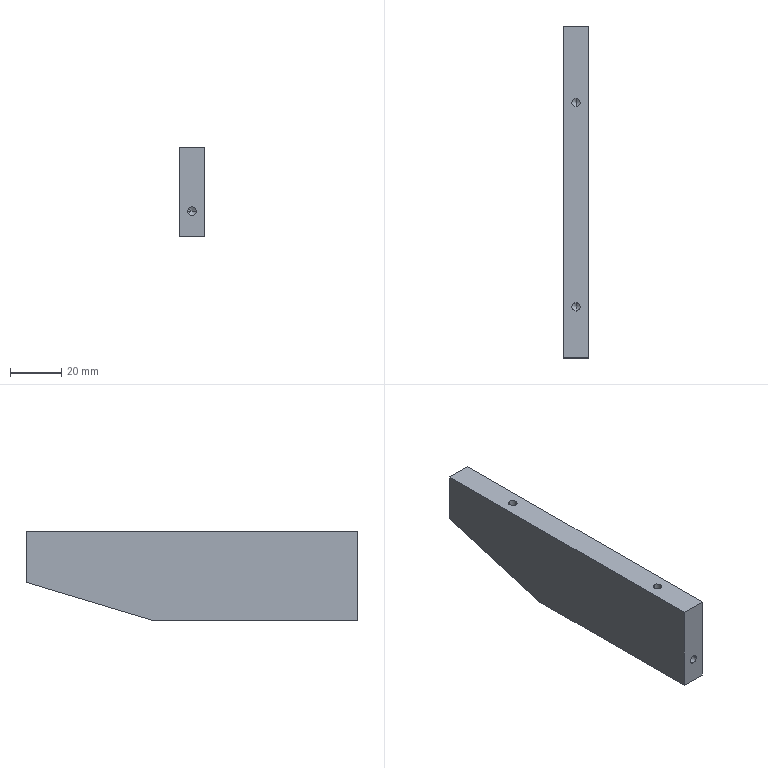Part | STEP file | 04-14 Guide reinforcing rib | 1 solid | 19 faces | box 10 x 130 x 35 mm | volume 41228 mm3 | plane 7 | cylinder 6 | cone 6 | commonest cylinder face diameters 3.3 x6
STEP:
#1=CARTESIAN_POINT('',(0.,0.,0.));
#2=DIRECTION('',(0.,0.,1.));
#3=DIRECTION('',(1.,0.,0.));
#4=AXIS2_PLACEMENT_3D('',#1,#2,#3);
#5=CARTESIAN_POINT('',(0.,18.35,-20.));
#6=VERTEX_POINT('',#5);
#7=CARTESIAN_POINT('',(0.,18.35,0.));
#8=VERTEX_POINT('',#7);
#9=CARTESIAN_POINT('',(0.,18.35,-20.));
#10=DIRECTION('',(0.,0.,1.));
#11=VECTOR('',#10,1.);
#12=LINE('',#9,#11);
#13=CARTESIAN_POINT('',(0.,20.,-20.));
#14=DIRECTION('',(0.,0.,1.));
#15=DIRECTION('',(0.,-1.,0.));
#16=AXIS2_PLACEMENT_3D('',#13,#14,#15);
#17=CYLINDRICAL_SURFACE('',#16,1.65);
#18=CARTESIAN_POINT('',(6.283,0.));
#19=DIRECTION('',(0.,1.));
#20=VECTOR('',#19,1.);
#21=LINE('',#18,#20);
#22=(GEOMETRIC_REPRESENTATION_CONTEXT(2)PARAMETRIC_REPRESENTATION_CONTEXT()REPRESENTATION_CONTEXT('',''));
#23=DEFINITIONAL_REPRESENTATION('',(#21),#22);
#24=PCURVE('',#17,#23);
#25=CARTESIAN_POINT('',(0.,20.,-20.));
#26=DIRECTION('',(0.,0.,1.));
#27=DIRECTION('',(0.,-1.,0.));
#28=AXIS2_PLACEMENT_3D('',#25,#26,#27);
#29=CYLINDRICAL_SURFACE('',#28,1.65);
#30=CARTESIAN_POINT('',(0.,0.));
#31=DIRECTION('',(0.,1.));
#32=VECTOR('',#31,1.);
#33=LINE('',#30,#32);
#34=(GEOMETRIC_REPRESENTATION_CONTEXT(2)PARAMETRIC_REPRESENTATION_CONTEXT()REPRESENTATION_CONTEXT('',''));
#35=DEFINITIONAL_REPRESENTATION('',(#33),#34);
#36=PCURVE('',#29,#35);
#37=SURFACE_CURVE('',#12,(#24,#36),.PCURVE_S1.);
#38=EDGE_CURVE('',#6,#8,#37,.T.);
#39=ORIENTED_EDGE('',*,*,#38,.T.);
#40=CARTESIAN_POINT('',(0.,21.65,0.));
#41=VERTEX_POINT('',#40);
#42=CARTESIAN_POINT('',(0.,20.,0.));
#43=DIRECTION('',(0.,0.,1.));
#44=DIRECTION('',(0.,-1.,0.));
#45=AXIS2_PLACEMENT_3D('',#42,#43,#44);
#46=CIRCLE('',#45,1.65);
#47=CARTESIAN_POINT('',(0.,20.));
#48=DIRECTION('',(1.,0.));
#49=VECTOR('',#48,1.);
#50=LINE('',#47,#49);
#51=(GEOMETRIC_REPRESENTATION_CONTEXT(2)PARAMETRIC_REPRESENTATION_CONTEXT()REPRESENTATION_CONTEXT('',''));
#52=DEFINITIONAL_REPRESENTATION('',(#50),#51);
#53=PCURVE('',#17,#52);
#54=CARTESIAN_POINT('',(5.,0.,0.));
#55=DIRECTION('',(0.,0.,-1.));
#56=DIRECTION('',(-1.,0.,0.));
#57=AXIS2_PLACEMENT_3D('',#54,#55,#56);
#58=PLANE('',#57);
#59=CARTESIAN_POINT('',(5.,18.35));
#60=CARTESIAN_POINT('',(2.142,18.35));
#61=CARTESIAN_POINT('',(3.571,20.825));
#62=CARTESIAN_POINT('',(5.,23.3));
#63=CARTESIAN_POINT('',(6.429,20.825));
#64=CARTESIAN_POINT('',(7.858,18.35));
#65=CARTESIAN_POINT('',(5.,18.35));
#66=(BOUNDED_CURVE()B_SPLINE_CURVE(2,(#59,#60,#61,#62,#63,#64,#65),.UNSPECIFIED.,.T.,.F.)B_SPLINE_CURVE_WITH_KNOTS((1,2,2,2,2,1),(-2.094,0.,2.094,4.189,6.283,8.378),.UNSPECIFIED.)CURVE()GEOMETRIC_REPRESENTATION_ITEM()RATIONAL_B_SPLINE_CURVE((1.,0.5,1.,0.5,1.,0.5,1.))REPRESENTATION_ITEM(''));
#67=(GEOMETRIC_REPRESENTATION_CONTEXT(2)PARAMETRIC_REPRESENTATION_CONTEXT()REPRESENTATION_CONTEXT('',''));
#68=DEFINITIONAL_REPRESENTATION('',(#66),#67);
#69=PCURVE('',#58,#68);
#70=SURFACE_CURVE('',#46,(#53,#69),.PCURVE_S1.);
#71=EDGE_CURVE('',#41,#8,#70,.T.);
#72=ORIENTED_EDGE('',*,*,#71,.F.);
#73=CARTESIAN_POINT('',(0.,21.65,-20.));
#74=VERTEX_POINT('',#73);
#75=CARTESIAN_POINT('',(0.,21.65,-20.));
#76=DIRECTION('',(0.,0.,1.));
#77=VECTOR('',#76,1.);
#78=LINE('',#75,#77);
#79=CARTESIAN_POINT('',(3.142,0.));
#80=DIRECTION('',(0.,1.));
#81=VECTOR('',#80,1.);
#82=LINE('',#79,#81);
#83=(GEOMETRIC_REPRESENTATION_CONTEXT(2)PARAMETRIC_REPRESENTATION_CONTEXT()REPRESENTATION_CONTEXT('',''));
#84=DEFINITIONAL_REPRESENTATION('',(#82),#83);
#85=PCURVE('',#17,#84);
#86=CARTESIAN_POINT('',(3.142,0.));
#87=DIRECTION('',(0.,1.));
#88=VECTOR('',#87,1.);
#89=LINE('',#86,#88);
#90=(GEOMETRIC_REPRESENTATION_CONTEXT(2)PARAMETRIC_REPRESENTATION_CONTEXT()REPRESENTATION_CONTEXT('',''));
#91=DEFINITIONAL_REPRESENTATION('',(#89),#90);
#92=PCURVE('',#29,#91);
#93=SURFACE_CURVE('',#78,(#85,#92),.PCURVE_S1.);
#94=EDGE_CURVE('',#74,#41,#93,.T.);
#95=ORIENTED_EDGE('',*,*,#94,.F.);
#96=CARTESIAN_POINT('',(0.,20.,-20.));
#97=DIRECTION('',(0.,0.,-1.));
#98=DIRECTION('',(1.,0.,0.));
#99=AXIS2_PLACEMENT_3D('',#96,#97,#98);
#100=CIRCLE('',#99,1.65);
#101=CARTESIAN_POINT('',(7.854,0.));
#102=DIRECTION('',(-1.,0.));
#103=VECTOR('',#102,1.);
#104=LINE('',#101,#103);
#105=(GEOMETRIC_REPRESENTATION_CONTEXT(2)PARAMETRIC_REPRESENTATION_CONTEXT()REPRESENTATION_CONTEXT('',''));
#106=DEFINITIONAL_REPRESENTATION('',(#104),#105);
#107=PCURVE('',#17,#106);
#108=CARTESIAN_POINT('',(0.,20.,979.009));
#109=DIRECTION('',(0.,0.,1.));
#110=DIRECTION('',(0.,-1.,0.));
#111=AXIS2_PLACEMENT_3D('',#108,#109,#110);
#112=CONICAL_SURFACE('',#111,1664.279,1.03);
#113=CARTESIAN_POINT('',(7.854,-999.009));
#114=DIRECTION('',(-1.,0.));
#115=VECTOR('',#114,1.);
#116=LINE('',#113,#115);
#117=(GEOMETRIC_REPRESENTATION_CONTEXT(2)PARAMETRIC_REPRESENTATION_CONTEXT()REPRESENTATION_CONTEXT('',''));
#118=DEFINITIONAL_REPRESENTATION('',(#116),#117);
#119=PCURVE('',#112,#118);
#120=SURFACE_CURVE('',#100,(#107,#119),.PCURVE_S1.);
#121=EDGE_CURVE('',#6,#74,#120,.T.);
#122=ORIENTED_EDGE('',*,*,#121,.F.);
#123=EDGE_LOOP('',(#39,#72,#95,#122));
#124=FACE_BOUND('',#123,.F.);
#125=ADVANCED_FACE('',(#124),#17,.F.);
#126=ORIENTED_EDGE('',*,*,#121,.T.);
#127=CARTESIAN_POINT('',(0.,20.,-20.991));
#128=VERTEX_POINT('',#127);
#129=CARTESIAN_POINT('',(0.,20.,-20.991));
#130=DIRECTION('',(0.,0.8572,0.515));
#131=VECTOR('',#130,1.);
#132=LINE('',#129,#131);
#133=CARTESIAN_POINT('',(3.142,-1000.));
#134=CARTESIAN_POINT('',(3.142,-999.985));
#135=CARTESIAN_POINT('',(3.142,-999.955));
#136=CARTESIAN_POINT('',(3.142,-999.91));
#137=CARTESIAN_POINT('',(3.142,-999.865));
#138=CARTESIAN_POINT('',(3.142,-999.82));
#139=CARTESIAN_POINT('',(3.142,-999.775));
#140=CARTESIAN_POINT('',(3.142,-999.73));
#141=CARTESIAN_POINT('',(3.142,-999.685));
#142=CARTESIAN_POINT('',(3.142,-999.639));
#143=CARTESIAN_POINT('',(3.142,-999.594));
#144=CARTESIAN_POINT('',(3.142,-999.549));
#145=CARTESIAN_POINT('',(3.142,-999.504));
#146=CARTESIAN_POINT('',(3.142,-999.459));
#147=CARTESIAN_POINT('',(3.142,-999.414));
#148=CARTESIAN_POINT('',(3.142,-999.369));
#149=CARTESIAN_POINT('',(3.142,-999.324));
#150=CARTESIAN_POINT('',(3.142,-999.279));
#151=CARTESIAN_POINT('',(3.142,-999.234));
#152=CARTESIAN_POINT('',(3.142,-999.189));
#153=CARTESIAN_POINT('',(3.142,-999.144));
#154=CARTESIAN_POINT('',(3.142,-999.099));
#155=CARTESIAN_POINT('',(3.142,-999.054));
#156=CARTESIAN_POINT('',(3.142,-999.024));
#157=CARTESIAN_POINT('',(3.142,-999.009));
#158=B_SPLINE_CURVE_WITH_KNOTS('',3,(#133,#134,#135,#136,#137,#138,#139,#140,#141,#142,#143,#144,#145,#146,#147,#148,#149,#150,#151,#152,#153,#154,#155,#156,#157),.UNSPECIFIED.,.F.,.F.,(4,1,1,1,1,1,1,1,1,1,1,1,1,1,1,1,1,1,1,1,1,1,4),(0.,0.0875,0.175,0.2625,0.35,0.4375,0.525,0.6125,0.7,0.7875,0.875,0.9625,1.05,1.137,1.225,1.312,1.4,1.487,1.575,1.662,1.75,1.837,1.925),.QUASI_UNIFORM_KNOTS.);
#159=(GEOMETRIC_REPRESENTATION_CONTEXT(2)PARAMETRIC_REPRESENTATION_CONTEXT()REPRESENTATION_CONTEXT('',''));
#160=DEFINITIONAL_REPRESENTATION('',(#158),#159);
#161=PCURVE('',#112,#160);
#162=CARTESIAN_POINT('',(0.,20.,979.009));
#163=DIRECTION('',(0.,0.,1.));
#164=DIRECTION('',(0.,-1.,0.));
#165=AXIS2_PLACEMENT_3D('',#162,#163,#164);
#166=CONICAL_SURFACE('',#165,1664.279,1.03);
#167=CARTESIAN_POINT('',(3.142,-1000.));
#168=CARTESIAN_POINT('',(3.142,-999.985));
#169=CARTESIAN_POINT('',(3.142,-999.955));
#170=CARTESIAN_POINT('',(3.142,-999.91));
#171=CARTESIAN_POINT('',(3.142,-999.865));
#172=CARTESIAN_POINT('',(3.142,-999.82));
#173=CARTESIAN_POINT('',(3.142,-999.775));
#174=CARTESIAN_POINT('',(3.142,-999.73));
#175=CARTESIAN_POINT('',(3.142,-999.685));
#176=CARTESIAN_POINT('',(3.142,-999.639));
#177=CARTESIAN_POINT('',(3.142,-999.594));
#178=CARTESIAN_POINT('',(3.142,-999.549));
#179=CARTESIAN_POINT('',(3.142,-999.504));
#180=CARTESIAN_POINT('',(3.142,-999.459));
#181=CARTESIAN_POINT('',(3.142,-999.414));
#182=CARTESIAN_POINT('',(3.142,-999.369));
#183=CARTESIAN_POINT('',(3.142,-999.324));
#184=CARTESIAN_POINT('',(3.142,-999.279));
#185=CARTESIAN_POINT('',(3.142,-999.234));
#186=CARTESIAN_POINT('',(3.142,-999.189));
#187=CARTESIAN_POINT('',(3.142,-999.144));
#188=CARTESIAN_POINT('',(3.142,-999.099));
#189=CARTESIAN_POINT('',(3.142,-999.054));
#190=CARTESIAN_POINT('',(3.142,-999.024));
#191=CARTESIAN_POINT('',(3.142,-999.009));
#192=B_SPLINE_CURVE_WITH_KNOTS('',3,(#167,#168,#169,#170,#171,#172,#173,#174,#175,#176,#177,#178,#179,#180,#181,#182,#183,#184,#185,#186,#187,#188,#189,#190,#191),.UNSPECIFIED.,.F.,.F.,(4,1,1,1,1,1,1,1,1,1,1,1,1,1,1,1,1,1,1,1,1,1,4),(0.,0.0875,0.175,0.2625,0.35,0.4375,0.525,0.6125,0.7,0.7875,0.875,0.9625,1.05,1.137,1.225,1.312,1.4,1.487,1.575,1.662,1.75,1.837,1.925),.QUASI_UNIFORM_KNOTS.);
#193=(GEOMETRIC_REPRESENTATION_CONTEXT(2)PARAMETRIC_REPRESENTATION_CONTEXT()REPRESENTATION_CONTEXT('',''));
#194=DEFINITIONAL_REPRESENTATION('',(#192),#193);
#195=PCURVE('',#166,#194);
#196=SURFACE_CURVE('',#132,(#161,#195),.PCURVE_S1.);
#197=EDGE_CURVE('',#128,#74,#196,.T.);
#198=ORIENTED_EDGE('',*,*,#197,.F.);
#199=CARTESIAN_POINT('',(0.,20.,-20.991));
#200=DIRECTION('',(0.,-0.8572,0.515));
#201=VECTOR('',#200,1.);
#202=LINE('',#199,#201);
#203=CARTESIAN_POINT('',(6.283,-1000.));
#204=DIRECTION('',(0.,1.));
#205=VECTOR('',#204,1.);
#206=LINE('',#203,#205);
#207=(GEOMETRIC_REPRESENTATION_CONTEXT(2)PARAMETRIC_REPRESENTATION_CONTEXT()REPRESENTATION_CONTEXT('',''));
#208=DEFINITIONAL_REPRESENTATION('',(#206),#207);
#209=PCURVE('',#112,#208);
#210=CARTESIAN_POINT('',(0.,-1000.));
#211=DIRECTION('',(0.,1.));
#212=VECTOR('',#211,1.);
#213=LINE('',#210,#212);
#214=(GEOMETRIC_REPRESENTATION_CONTEXT(2)PARAMETRIC_REPRESENTATION_CONTEXT()REPRESENTATION_CONTEXT('',''));
#215=DEFINITIONAL_REPRESENTATION('',(#213),#214);
#216=PCURVE('',#166,#215);
#217=SURFACE_CURVE('',#202,(#209,#216),.PCURVE_S1.);
#218=EDGE_CURVE('',#128,#6,#217,.T.);
#219=ORIENTED_EDGE('',*,*,#218,.T.);
#220=EDGE_LOOP('',(#126,#198,#219));
#221=FACE_BOUND('',#220,.F.);
#222=ADVANCED_FACE('',(#221),#112,.F.);
#223=CARTESIAN_POINT('',(0.,98.35,-20.));
#224=VERTEX_POINT('',#223);
#225=CARTESIAN_POINT('',(0.,98.35,0.));
#226=VERTEX_POINT('',#225);
#227=CARTESIAN_POINT('',(0.,98.35,-20.));
#228=DIRECTION('',(0.,0.,1.));
#229=VECTOR('',#228,1.);
#230=LINE('',#227,#229);
#231=CARTESIAN_POINT('',(0.,100.,-20.));
#232=DIRECTION('',(0.,0.,1.));
#233=DIRECTION('',(0.,-1.,0.));
#234=AXIS2_PLACEMENT_3D('',#231,#232,#233);
#235=CYLINDRICAL_SURFACE('',#234,1.65);
#236=CARTESIAN_POINT('',(6.283,0.));
#237=DIRECTION('',(0.,1.));
#238=VECTOR('',#237,1.);
#239=LINE('',#236,#238);
#240=(GEOMETRIC_REPRESENTATION_CONTEXT(2)PARAMETRIC_REPRESENTATION_CONTEXT()REPRESENTATION_CONTEXT('',''));
#241=DEFINITIONAL_REPRESENTATION('',(#239),#240);
#242=PCURVE('',#235,#241);
#243=CARTESIAN_POINT('',(0.,100.,-20.));
#244=DIRECTION('',(0.,0.,1.));
#245=DIRECTION('',(0.,-1.,0.));
#246=AXIS2_PLACEMENT_3D('',#243,#244,#245);
#247=CYLINDRICAL_SURFACE('',#246,1.65);
#248=CARTESIAN_POINT('',(0.,0.));
#249=DIRECTION('',(0.,1.));
#250=VECTOR('',#249,1.);
#251=LINE('',#248,#250);
#252=(GEOMETRIC_REPRESENTATION_CONTEXT(2)PARAMETRIC_REPRESENTATION_CONTEXT()REPRESENTATION_CONTEXT('',''));
#253=DEFINITIONAL_REPRESENTATION('',(#251),#252);
#254=PCURVE('',#247,#253);
#255=SURFACE_CURVE('',#230,(#242,#254),.PCURVE_S1.);
#256=EDGE_CURVE('',#224,#226,#255,.T.);
#257=ORIENTED_EDGE('',*,*,#256,.T.);
#258=CARTESIAN_POINT('',(0.,101.65,0.));
#259=VERTEX_POINT('',#258);
#260=CARTESIAN_POINT('',(0.,100.,0.));
#261=DIRECTION('',(0.,0.,1.));
#262=DIRECTION('',(0.,-1.,0.));
#263=AXIS2_PLACEMENT_3D('',#260,#261,#262);
#264=CIRCLE('',#263,1.65);
#265=CARTESIAN_POINT('',(0.,20.));
#266=DIRECTION('',(1.,0.));
#267=VECTOR('',#266,1.);
#268=LINE('',#265,#267);
#269=(GEOMETRIC_REPRESENTATION_CONTEXT(2)PARAMETRIC_REPRESENTATION_CONTEXT()REPRESENTATION_CONTEXT('',''));
#270=DEFINITIONAL_REPRESENTATION('',(#268),#269);
#271=PCURVE('',#235,#270);
#272=CARTESIAN_POINT('',(5.,98.35));
#273=CARTESIAN_POINT('',(2.142,98.35));
#274=CARTESIAN_POINT('',(3.571,100.825));
#275=CARTESIAN_POINT('',(5.,103.3));
#276=CARTESIAN_POINT('',(6.429,100.825));
#277=CARTESIAN_POINT('',(7.858,98.35));
#278=CARTESIAN_POINT('',(5.,98.35));
#279=(BOUNDED_CURVE()B_SPLINE_CURVE(2,(#272,#273,#274,#275,#276,#277,#278),.UNSPECIFIED.,.T.,.F.)B_SPLINE_CURVE_WITH_KNOTS((1,2,2,2,2,1),(-2.094,0.,2.094,4.189,6.283,8.378),.UNSPECIFIED.)CURVE()GEOMETRIC_REPRESENTATION_ITEM()RATIONAL_B_SPLINE_CURVE((1.,0.5,1.,0.5,1.,0.5,1.))REPRESENTATION_ITEM(''));
#280=(GEOMETRIC_REPRESENTATION_CONTEXT(2)PARAMETRIC_REPRESENTATION_CONTEXT()REPRESENTATION_CONTEXT('',''));
#281=DEFINITIONAL_REPRESENTATION('',(#279),#280);
#282=PCURVE('',#58,#281);
#283=SURFACE_CURVE('',#264,(#271,#282),.PCURVE_S1.);
#284=EDGE_CURVE('',#259,#226,#283,.T.);
#285=ORIENTED_EDGE('',*,*,#284,.F.);
#286=CARTESIAN_POINT('',(0.,101.65,-20.));
#287=VERTEX_POINT('',#286);
#288=CARTESIAN_POINT('',(0.,101.65,-20.));
#289=DIRECTION('',(0.,0.,1.));
#290=VECTOR('',#289,1.);
#291=LINE('',#288,#290);
#292=CARTESIAN_POINT('',(3.142,0.));
#293=DIRECTION('',(0.,1.));
#294=VECTOR('',#293,1.);
#295=LINE('',#292,#294);
#296=(GEOMETRIC_REPRESENTATION_CONTEXT(2)PARAMETRIC_REPRESENTATION_CONTEXT()REPRESENTATION_CONTEXT('',''));
#297=DEFINITIONAL_REPRESENTATION('',(#295),#296);
#298=PCURVE('',#235,#297);
#299=CARTESIAN_POINT('',(3.142,0.));
#300=DIRECTION('',(0.,1.));
#301=VECTOR('',#300,1.);
#302=LINE('',#299,#301);
#303=(GEOMETRIC_REPRESENTATION_CONTEXT(2)PARAMETRIC_REPRESENTATION_CONTEXT()REPRESENTATION_CONTEXT('',''));
#304=DEFINITIONAL_REPRESENTATION('',(#302),#303);
#305=PCURVE('',#247,#304);
#306=SURFACE_CURVE('',#291,(#298,#305),.PCURVE_S1.);
#307=EDGE_CURVE('',#287,#259,#306,.T.);
#308=ORIENTED_EDGE('',*,*,#307,.F.);
#309=CARTESIAN_POINT('',(0.,100.,-20.));
#310=DIRECTION('',(0.,0.,-1.));
#311=DIRECTION('',(1.,0.,0.));
#312=AXIS2_PLACEMENT_3D('',#309,#310,#311);
#313=CIRCLE('',#312,1.65);
#314=CARTESIAN_POINT('',(7.854,0.));
#315=DIRECTION('',(-1.,0.));
#316=VECTOR('',#315,1.);
#317=LINE('',#314,#316);
#318=(GEOMETRIC_REPRESENTATION_CONTEXT(2)PARAMETRIC_REPRESENTATION_CONTEXT()REPRESENTATION_CONTEXT('',''));
#319=DEFINITIONAL_REPRESENTATION('',(#317),#318);
#320=PCURVE('',#235,#319);
#321=CARTESIAN_POINT('',(0.,100.,979.009));
#322=DIRECTION('',(0.,0.,1.));
#323=DIRECTION('',(0.,-1.,0.));
#324=AXIS2_PLACEMENT_3D('',#321,#322,#323);
#325=CONICAL_SURFACE('',#324,1664.279,1.03);
#326=CARTESIAN_POINT('',(7.854,-999.009));
#327=DIRECTION('',(-1.,0.));
#328=VECTOR('',#327,1.);
#329=LINE('',#326,#328);
#330=(GEOMETRIC_REPRESENTATION_CONTEXT(2)PARAMETRIC_REPRESENTATION_CONTEXT()REPRESENTATION_CONTEXT('',''));
#331=DEFINITIONAL_REPRESENTATION('',(#329),#330);
#332=PCURVE('',#325,#331);
#333=SURFACE_CURVE('',#313,(#320,#332),.PCURVE_S1.);
#334=EDGE_CURVE('',#224,#287,#333,.T.);
#335=ORIENTED_EDGE('',*,*,#334,.F.);
#336=EDGE_LOOP('',(#257,#285,#308,#335));
#337=FACE_BOUND('',#336,.F.);
#338=ADVANCED_FACE('',(#337),#235,.F.);
#339=ORIENTED_EDGE('',*,*,#334,.T.);
#340=CARTESIAN_POINT('',(0.,100.,-20.991));
#341=VERTEX_POINT('',#340);
#342=CARTESIAN_POINT('',(0.,100.,-20.991));
#343=DIRECTION('',(0.,0.8572,0.515));
#344=VECTOR('',#343,1.);
#345=LINE('',#342,#344);
#346=CARTESIAN_POINT('',(3.142,-1000.));
#347=CARTESIAN_POINT('',(3.142,-999.985));
#348=CARTESIAN_POINT('',(3.142,-999.955));
#349=CARTESIAN_POINT('',(3.142,-999.91));
#350=CARTESIAN_POINT('',(3.142,-999.865));
#351=CARTESIAN_POINT('',(3.142,-999.82));
#352=CARTESIAN_POINT('',(3.142,-999.775));
#353=CARTESIAN_POINT('',(3.142,-999.73));
#354=CARTESIAN_POINT('',(3.142,-999.685));
#355=CARTESIAN_POINT('',(3.142,-999.639));
#356=CARTESIAN_POINT('',(3.142,-999.594));
#357=CARTESIAN_POINT('',(3.142,-999.549));
#358=CARTESIAN_POINT('',(3.142,-999.504));
#359=CARTESIAN_POINT('',(3.142,-999.459));
#360=CARTESIAN_POINT('',(3.142,-999.414));
#361=CARTESIAN_POINT('',(3.142,-999.369));
#362=CARTESIAN_POINT('',(3.142,-999.324));
#363=CARTESIAN_POINT('',(3.142,-999.279));
#364=CARTESIAN_POINT('',(3.142,-999.234));
#365=CARTESIAN_POINT('',(3.142,-999.189));
#366=CARTESIAN_POINT('',(3.142,-999.144));
#367=CARTESIAN_POINT('',(3.142,-999.099));
#368=CARTESIAN_POINT('',(3.142,-999.054));
#369=CARTESIAN_POINT('',(3.142,-999.024));
#370=CARTESIAN_POINT('',(3.142,-999.009));
#371=B_SPLINE_CURVE_WITH_KNOTS('',3,(#346,#347,#348,#349,#350,#351,#352,#353,#354,#355,#356,#357,#358,#359,#360,#361,#362,#363,#364,#365,#366,#367,#368,#369,#370),.UNSPECIFIED.,.F.,.F.,(4,1,1,1,1,1,1,1,1,1,1,1,1,1,1,1,1,1,1,1,1,1,4),(0.,0.0875,0.175,0.2625,0.35,0.4375,0.525,0.6125,0.7,0.7875,0.875,0.9625,1.05,1.137,1.225,1.312,1.4,1.487,1.575,1.662,1.75,1.837,1.925),.QUASI_UNIFORM_KNOTS.);
#372=(GEOMETRIC_REPRESENTATION_CONTEXT(2)PARAMETRIC_REPRESENTATION_CONTEXT()REPRESENTATION_CONTEXT('',''));
#373=DEFINITIONAL_REPRESENTATION('',(#371),#372);
#374=PCURVE('',#325,#373);
#375=CARTESIAN_POINT('',(0.,100.,979.009));
#376=DIRECTION('',(0.,0.,1.));
#377=DIRECTION('',(0.,-1.,0.));
#378=AXIS2_PLACEMENT_3D('',#375,#376,#377);
#379=CONICAL_SURFACE('',#378,1664.279,1.03);
#380=CARTESIAN_POINT('',(3.142,-1000.));
#381=CARTESIAN_POINT('',(3.142,-999.985));
#382=CARTESIAN_POINT('',(3.142,-999.955));
#383=CARTESIAN_POINT('',(3.142,-999.91));
#384=CARTESIAN_POINT('',(3.142,-999.865));
#385=CARTESIAN_POINT('',(3.142,-999.82));
#386=CARTESIAN_POINT('',(3.142,-999.775));
#387=CARTESIAN_POINT('',(3.142,-999.73));
#388=CARTESIAN_POINT('',(3.142,-999.685));
#389=CARTESIAN_POINT('',(3.142,-999.639));
#390=CARTESIAN_POINT('',(3.142,-999.594));
#391=CARTESIAN_POINT('',(3.142,-999.549));
#392=CARTESIAN_POINT('',(3.142,-999.504));
#393=CARTESIAN_POINT('',(3.142,-999.459));
#394=CARTESIAN_POINT('',(3.142,-999.414));
#395=CARTESIAN_POINT('',(3.142,-999.369));
#396=CARTESIAN_POINT('',(3.142,-999.324));
#397=CARTESIAN_POINT('',(3.142,-999.279));
#398=CARTESIAN_POINT('',(3.142,-999.234));
#399=CARTESIAN_POINT('',(3.142,-999.189));
#400=CARTESIAN_POINT('',(3.142,-999.144));
#401=CARTESIAN_POINT('',(3.142,-999.099));
#402=CARTESIAN_POINT('',(3.142,-999.054));
#403=CARTESIAN_POINT('',(3.142,-999.024));
#404=CARTESIAN_POINT('',(3.142,-999.009));
#405=B_SPLINE_CURVE_WITH_KNOTS('',3,(#380,#381,#382,#383,#384,#385,#386,#387,#388,#389,#390,#391,#392,#393,#394,#395,#396,#397,#398,#399,#400,#401,#402,#403,#404),.UNSPECIFIED.,.F.,.F.,(4,1,1,1,1,1,1,1,1,1,1,1,1,1,1,1,1,1,1,1,1,1,4),(0.,0.0875,0.175,0.2625,0.35,0.4375,0.525,0.6125,0.7,0.7875,0.875,0.9625,1.05,1.137,1.225,1.312,1.4,1.487,1.575,1.662,1.75,1.837,1.925),.QUASI_UNIFORM_KNOTS.);
#406=(GEOMETRIC_REPRESENTATION_CONTEXT(2)PARAMETRIC_REPRESENTATION_CONTEXT()REPRESENTATION_CONTEXT('',''));
#407=DEFINITIONAL_REPRESENTATION('',(#405),#406);
#408=PCURVE('',#379,#407);
#409=SURFACE_CURVE('',#345,(#374,#408),.PCURVE_S1.);
#410=EDGE_CURVE('',#341,#287,#409,.T.);
#411=ORIENTED_EDGE('',*,*,#410,.F.);
#412=CARTESIAN_POINT('',(0.,100.,-20.991));
#413=DIRECTION('',(0.,-0.8572,0.515));
#414=VECTOR('',#413,1.);
#415=LINE('',#412,#414);
#416=CARTESIAN_POINT('',(6.283,-1000.));
#417=DIRECTION('',(0.,1.));
#418=VECTOR('',#417,1.);
#419=LINE('',#416,#418);
#420=(GEOMETRIC_REPRESENTATION_CONTEXT(2)PARAMETRIC_REPRESENTATION_CONTEXT()REPRESENTATION_CONTEXT('',''));
#421=DEFINITIONAL_REPRESENTATION('',(#419),#420);
#422=PCURVE('',#325,#421);
#423=CARTESIAN_POINT('',(0.,-1000.));
#424=DIRECTION('',(0.,1.));
#425=VECTOR('',#424,1.);
#426=LINE('',#423,#425);
#427=(GEOMETRIC_REPRESENTATION_CONTEXT(2)PARAMETRIC_REPRESENTATION_CONTEXT()REPRESENTATION_CONTEXT('',''));
#428=DEFINITIONAL_REPRESENTATION('',(#426),#427);
#429=PCURVE('',#379,#428);
#430=SURFACE_CURVE('',#415,(#422,#429),.PCURVE_S1.);
#431=EDGE_CURVE('',#341,#224,#430,.T.);
#432=ORIENTED_EDGE('',*,*,#431,.T.);
#433=EDGE_LOOP('',(#339,#411,#432));
#434=FACE_BOUND('',#433,.F.);
#435=ADVANCED_FACE('',(#434),#325,.F.);
#436=CARTESIAN_POINT('',(1.65,20.,-25.));
#437=VERTEX_POINT('',#436);
#438=CARTESIAN_POINT('',(1.65,0.,-25.));
#439=VERTEX_POINT('',#438);
#440=CARTESIAN_POINT('',(1.65,20.,-25.));
#441=DIRECTION('',(0.,-1.,0.));
#442=VECTOR('',#441,1.);
#443=LINE('',#440,#442);
#444=CARTESIAN_POINT('',(0.,20.,-25.));
#445=DIRECTION('',(0.,-1.,0.));
#446=DIRECTION('',(1.,0.,0.));
#447=AXIS2_PLACEMENT_3D('',#444,#445,#446);
#448=CYLINDRICAL_SURFACE('',#447,1.65);
#449=CARTESIAN_POINT('',(6.283,0.));
#450=DIRECTION('',(0.,1.));
#451=VECTOR('',#450,1.);
#452=LINE('',#449,#451);
#453=(GEOMETRIC_REPRESENTATION_CONTEXT(2)PARAMETRIC_REPRESENTATION_CONTEXT()REPRESENTATION_CONTEXT('',''));
#454=DEFINITIONAL_REPRESENTATION('',(#452),#453);
#455=PCURVE('',#448,#454);
#456=CARTESIAN_POINT('',(0.,20.,-25.));
#457=DIRECTION('',(0.,-1.,0.));
#458=DIRECTION('',(1.,0.,0.));
#459=AXIS2_PLACEMENT_3D('',#456,#457,#458);
#460=CYLINDRICAL_SURFACE('',#459,1.65);
#461=CARTESIAN_POINT('',(0.,0.));
#462=DIRECTION('',(0.,1.));
#463=VECTOR('',#462,1.);
#464=LINE('',#461,#463);
#465=(GEOMETRIC_REPRESENTATION_CONTEXT(2)PARAMETRIC_REPRESENTATION_CONTEXT()REPRESENTATION_CONTEXT('',''));
#466=DEFINITIONAL_REPRESENTATION('',(#464),#465);
#467=PCURVE('',#460,#466);
#468=SURFACE_CURVE('',#443,(#455,#467),.PCURVE_S1.);
#469=EDGE_CURVE('',#437,#439,#468,.T.);
#470=ORIENTED_EDGE('',*,*,#469,.T.);
#471=CARTESIAN_POINT('',(-1.65,0.,-25.));
#472=VERTEX_POINT('',#471);
#473=CARTESIAN_POINT('',(0.,0.,-25.));
#474=DIRECTION('',(0.,-1.,0.));
#475=DIRECTION('',(1.,0.,0.));
#476=AXIS2_PLACEMENT_3D('',#473,#474,#475);
#477=CIRCLE('',#476,1.65);
#478=CARTESIAN_POINT('',(0.,20.));
#479=DIRECTION('',(1.,0.));
#480=VECTOR('',#479,1.);
#481=LINE('',#478,#480);
#482=(GEOMETRIC_REPRESENTATION_CONTEXT(2)PARAMETRIC_REPRESENTATION_CONTEXT()REPRESENTATION_CONTEXT('',''));
#483=DEFINITIONAL_REPRESENTATION('',(#481),#482);
#484=PCURVE('',#448,#483);
#485=CARTESIAN_POINT('',(-5.,0.,-35.));
#486=DIRECTION('',(0.,1.,0.));
#487=DIRECTION('',(0.,0.,1.));
#488=AXIS2_PLACEMENT_3D('',#485,#486,#487);
#489=PLANE('',#488);
#490=CARTESIAN_POINT('',(10.,6.65));
#491=CARTESIAN_POINT('',(12.858,6.65));
#492=CARTESIAN_POINT('',(11.429,4.175));
#493=CARTESIAN_POINT('',(10.,1.7));
#494=CARTESIAN_POINT('',(8.571,4.175));
#495=CARTESIAN_POINT('',(7.142,6.65));
#496=CARTESIAN_POINT('',(10.,6.65));
#497=(BOUNDED_CURVE()B_SPLINE_CURVE(2,(#490,#491,#492,#493,#494,#495,#496),.UNSPECIFIED.,.T.,.F.)B_SPLINE_CURVE_WITH_KNOTS((1,2,2,2,2,1),(-2.094,0.,2.094,4.189,6.283,8.378),.UNSPECIFIED.)CURVE()GEOMETRIC_REPRESENTATION_ITEM()RATIONAL_B_SPLINE_CURVE((1.,0.5,1.,0.5,1.,0.5,1.))REPRESENTATION_ITEM(''));
#498=(GEOMETRIC_REPRESENTATION_CONTEXT(2)PARAMETRIC_REPRESENTATION_CONTEXT()REPRESENTATION_CONTEXT('',''));
#499=DEFINITIONAL_REPRESENTATION('',(#497),#498);
#500=PCURVE('',#489,#499);
#501=SURFACE_CURVE('',#477,(#484,#500),.PCURVE_S1.);
#502=EDGE_CURVE('',#472,#439,#501,.T.);
#503=ORIENTED_EDGE('',*,*,#502,.F.);
#504=CARTESIAN_POINT('',(-1.65,20.,-25.));
#505=VERTEX_POINT('',#504);
#506=CARTESIAN_POINT('',(-1.65,20.,-25.));
#507=DIRECTION('',(0.,-1.,0.));
#508=VECTOR('',#507,1.);
#509=LINE('',#506,#508);
#510=CARTESIAN_POINT('',(3.142,0.));
#511=DIRECTION('',(0.,1.));
#512=VECTOR('',#511,1.);
#513=LINE('',#510,#512);
#514=(GEOMETRIC_REPRESENTATION_CONTEXT(2)PARAMETRIC_REPRESENTATION_CONTEXT()REPRESENTATION_CONTEXT('',''));
#515=DEFINITIONAL_REPRESENTATION('',(#513),#514);
#516=PCURVE('',#448,#515);
#517=CARTESIAN_POINT('',(3.142,0.));
#518=DIRECTION('',(0.,1.));
#519=VECTOR('',#518,1.);
#520=LINE('',#517,#519);
#521=(GEOMETRIC_REPRESENTATION_CONTEXT(2)PARAMETRIC_REPRESENTATION_CONTEXT()REPRESENTATION_CONTEXT('',''));
#522=DEFINITIONAL_REPRESENTATION('',(#520),#521);
#523=PCURVE('',#460,#522);
#524=SURFACE_CURVE('',#509,(#516,#523),.PCURVE_S1.);
#525=EDGE_CURVE('',#505,#472,#524,.T.);
#526=ORIENTED_EDGE('',*,*,#525,.F.);
#527=CARTESIAN_POINT('',(0.,20.,-25.));
#528=DIRECTION('',(0.,1.,0.));
#529=DIRECTION('',(0.,0.,-1.));
#530=AXIS2_PLACEMENT_3D('',#527,#528,#529);
#531=CIRCLE('',#530,1.65);
#532=CARTESIAN_POINT('',(10.996,0.));
#533=DIRECTION('',(-1.,0.));
#534=VECTOR('',#533,1.);
#535=LINE('',#532,#534);
#536=(GEOMETRIC_REPRESENTATION_CONTEXT(2)PARAMETRIC_REPRESENTATION_CONTEXT()REPRESENTATION_CONTEXT('',''));
#537=DEFINITIONAL_REPRESENTATION('',(#535),#536);
#538=PCURVE('',#448,#537);
#539=CARTESIAN_POINT('',(0.,-979.009,-25.));
#540=DIRECTION('',(0.,-1.,0.));
#541=DIRECTION('',(1.,0.,0.));
#542=AXIS2_PLACEMENT_3D('',#539,#540,#541);
#543=CONICAL_SURFACE('',#542,1664.279,1.03);
#544=CARTESIAN_POINT('',(10.996,-999.009));
#545=DIRECTION('',(-1.,0.));
#546=VECTOR('',#545,1.);
#547=LINE('',#544,#546);
#548=(GEOMETRIC_REPRESENTATION_CONTEXT(2)PARAMETRIC_REPRESENTATION_CONTEXT()REPRESENTATION_CONTEXT('',''));
#549=DEFINITIONAL_REPRESENTATION('',(#547),#548);
#550=PCURVE('',#543,#549);
#551=SURFACE_CURVE('',#531,(#538,#550),.PCURVE_S1.);
#552=EDGE_CURVE('',#437,#505,#551,.T.);
#553=ORIENTED_EDGE('',*,*,#552,.F.);
#554=EDGE_LOOP('',(#470,#503,#526,#553));
#555=FACE_BOUND('',#554,.F.);
#556=ADVANCED_FACE('',(#555),#448,.F.);
#557=ORIENTED_EDGE('',*,*,#552,.T.);
#558=CARTESIAN_POINT('',(0.,20.991,-25.));
#559=VERTEX_POINT('',#558);
#560=CARTESIAN_POINT('',(0.,20.991,-25.));
#561=DIRECTION('',(-0.8572,-0.515,0.));
#562=VECTOR('',#561,1.);
#563=LINE('',#560,#562);
#564=CARTESIAN_POINT('',(3.142,-1000.));
#565=DIRECTION('',(0.,1.));
#566=VECTOR('',#565,1.);
#567=LINE('',#564,#566);
#568=(GEOMETRIC_REPRESENTATION_CONTEXT(2)PARAMETRIC_REPRESENTATION_CONTEXT()REPRESENTATION_CONTEXT('',''));
#569=DEFINITIONAL_REPRESENTATION('',(#567),#568);
#570=PCURVE('',#543,#569);
#571=CARTESIAN_POINT('',(0.,-979.009,-25.));
#572=DIRECTION('',(0.,-1.,0.));
#573=DIRECTION('',(1.,0.,0.));
#574=AXIS2_PLACEMENT_3D('',#571,#572,#573);
#575=CONICAL_SURFACE('',#574,1664.279,1.03);
#576=CARTESIAN_POINT('',(3.142,-1000.));
#577=DIRECTION('',(0.,1.));
#578=VECTOR('',#577,1.);
#579=LINE('',#576,#578);
#580=(GEOMETRIC_REPRESENTATION_CONTEXT(2)PARAMETRIC_REPRESENTATION_CONTEXT()REPRESENTATION_CONTEXT('',''));
#581=DEFINITIONAL_REPRESENTATION('',(#579),#580);
#582=PCURVE('',#575,#581);
#583=SURFACE_CURVE('',#563,(#570,#582),.PCURVE_S1.);
#584=EDGE_CURVE('',#559,#505,#583,.T.);
#585=ORIENTED_EDGE('',*,*,#584,.F.);
#586=CARTESIAN_POINT('',(0.,20.991,-25.));
#587=DIRECTION('',(0.8572,-0.515,0.));
#588=VECTOR('',#587,1.);
#589=LINE('',#586,#588);
#590=CARTESIAN_POINT('',(6.283,-1000.));
#591=CARTESIAN_POINT('',(6.283,-999.985));
#592=CARTESIAN_POINT('',(6.283,-999.955));
#593=CARTESIAN_POINT('',(6.283,-999.91));
#594=CARTESIAN_POINT('',(6.283,-999.865));
#595=CARTESIAN_POINT('',(6.283,-999.82));
#596=CARTESIAN_POINT('',(6.283,-999.775));
#597=CARTESIAN_POINT('',(6.283,-999.73));
#598=CARTESIAN_POINT('',(6.283,-999.685));
#599=CARTESIAN_POINT('',(6.283,-999.639));
#600=CARTESIAN_POINT('',(6.283,-999.594));
#601=CARTESIAN_POINT('',(6.283,-999.549));
#602=CARTESIAN_POINT('',(6.283,-999.504));
#603=CARTESIAN_POINT('',(6.283,-999.459));
#604=CARTESIAN_POINT('',(6.283,-999.414));
#605=CARTESIAN_POINT('',(6.283,-999.369));
#606=CARTESIAN_POINT('',(6.283,-999.324));
#607=CARTESIAN_POINT('',(6.283,-999.279));
#608=CARTESIAN_POINT('',(6.283,-999.234));
#609=CARTESIAN_POINT('',(6.283,-999.189));
#610=CARTESIAN_POINT('',(6.283,-999.144));
#611=CARTESIAN_POINT('',(6.283,-999.099));
#612=CARTESIAN_POINT('',(6.283,-999.054));
#613=CARTESIAN_POINT('',(6.283,-999.024));
#614=CARTESIAN_POINT('',(6.283,-999.009));
#615=B_SPLINE_CURVE_WITH_KNOTS('',3,(#590,#591,#592,#593,#594,#595,#596,#597,#598,#599,#600,#601,#602,#603,#604,#605,#606,#607,#608,#609,#610,#611,#612,#613,#614),.UNSPECIFIED.,.F.,.F.,(4,1,1,1,1,1,1,1,1,1,1,1,1,1,1,1,1,1,1,1,1,1,4),(0.,0.0875,0.175,0.2625,0.35,0.4375,0.525,0.6125,0.7,0.7875,0.875,0.9625,1.05,1.137,1.225,1.312,1.4,1.487,1.575,1.662,1.75,1.837,1.925),.QUASI_UNIFORM_KNOTS.);
#616=(GEOMETRIC_REPRESENTATION_CONTEXT(2)PARAMETRIC_REPRESENTATION_CONTEXT()REPRESENTATION_CONTEXT('',''));
#617=DEFINITIONAL_REPRESENTATION('',(#615),#616);
#618=PCURVE('',#543,#617);
#619=CARTESIAN_POINT('',(0.,-1000.));
#620=CARTESIAN_POINT('',(0.,-999.985));
#621=CARTESIAN_POINT('',(0.,-999.955));
#622=CARTESIAN_POINT('',(0.,-999.91));
#623=CARTESIAN_POINT('',(0.,-999.865));
#624=CARTESIAN_POINT('',(0.,-999.82));
#625=CARTESIAN_POINT('',(0.,-999.775));
#626=CARTESIAN_POINT('',(0.,-999.73));
#627=CARTESIAN_POINT('',(0.,-999.685));
#628=CARTESIAN_POINT('',(0.,-999.639));
#629=CARTESIAN_POINT('',(0.,-999.594));
#630=CARTESIAN_POINT('',(0.,-999.549));
#631=CARTESIAN_POINT('',(0.,-999.504));
#632=CARTESIAN_POINT('',(0.,-999.459));
#633=CARTESIAN_POINT('',(0.,-999.414));
#634=CARTESIAN_POINT('',(0.,-999.369));
#635=CARTESIAN_POINT('',(0.,-999.324));
#636=CARTESIAN_POINT('',(0.,-999.279));
#637=CARTESIAN_POINT('',(0.,-999.234));
#638=CARTESIAN_POINT('',(0.,-999.189));
#639=CARTESIAN_POINT('',(0.,-999.144));
#640=CARTESIAN_POINT('',(0.,-999.099));
#641=CARTESIAN_POINT('',(0.,-999.054));
#642=CARTESIAN_POINT('',(0.,-999.024));
#643=CARTESIAN_POINT('',(0.,-999.009));
#644=B_SPLINE_CURVE_WITH_KNOTS('',3,(#619,#620,#621,#622,#623,#624,#625,#626,#627,#628,#629,#630,#631,#632,#633,#634,#635,#636,#637,#638,#639,#640,#641,#642,#643),.UNSPECIFIED.,.F.,.F.,(4,1,1,1,1,1,1,1,1,1,1,1,1,1,1,1,1,1,1,1,1,1,4),(0.,0.0875,0.175,0.2625,0.35,0.4375,0.525,0.6125,0.7,0.7875,0.875,0.9625,1.05,1.137,1.225,1.312,1.4,1.487,1.575,1.662,1.75,1.837,1.925),.QUASI_UNIFORM_KNOTS.);
#645=(GEOMETRIC_REPRESENTATION_CONTEXT(2)PARAMETRIC_REPRESENTATION_CONTEXT()REPRESENTATION_CONTEXT('',''));
#646=DEFINITIONAL_REPRESENTATION('',(#644),#645);
#647=PCURVE('',#575,#646);
#648=SURFACE_CURVE('',#589,(#618,#647),.PCURVE_S1.);
#649=EDGE_CURVE('',#559,#437,#648,.T.);
#650=ORIENTED_EDGE('',*,*,#649,.T.);
#651=EDGE_LOOP('',(#557,#585,#650));
#652=FACE_BOUND('',#651,.F.);
#653=ADVANCED_FACE('',(#652),#543,.F.);
#654=CARTESIAN_POINT('',(0.,20.,0.));
#655=DIRECTION('',(0.,0.,1.));
#656=DIRECTION('',(0.,-1.,0.));
#657=AXIS2_PLACEMENT_3D('',#654,#655,#656);
#658=CIRCLE('',#657,1.65);
#659=CARTESIAN_POINT('',(0.,20.));
#660=DIRECTION('',(1.,0.));
#661=VECTOR('',#660,1.);
#662=LINE('',#659,#661);
#663=(GEOMETRIC_REPRESENTATION_CONTEXT(2)PARAMETRIC_REPRESENTATION_CONTEXT()REPRESENTATION_CONTEXT('',''));
#664=DEFINITIONAL_REPRESENTATION('',(#662),#663);
#665=PCURVE('',#29,#664);
#666=CARTESIAN_POINT('',(5.,18.35));
#667=CARTESIAN_POINT('',(2.142,18.35));
#668=CARTESIAN_POINT('',(3.571,20.825));
#669=CARTESIAN_POINT('',(5.,23.3));
#670=CARTESIAN_POINT('',(6.429,20.825));
#671=CARTESIAN_POINT('',(7.858,18.35));
#672=CARTESIAN_POINT('',(5.,18.35));
#673=(BOUNDED_CURVE()B_SPLINE_CURVE(2,(#666,#667,#668,#669,#670,#671,#672),.UNSPECIFIED.,.T.,.F.)B_SPLINE_CURVE_WITH_KNOTS((1,2,2,2,2,1),(-2.094,0.,2.094,4.189,6.283,8.378),.UNSPECIFIED.)CURVE()GEOMETRIC_REPRESENTATION_ITEM()RATIONAL_B_SPLINE_CURVE((1.,0.5,1.,0.5,1.,0.5,1.))REPRESENTATION_ITEM(''));
#674=(GEOMETRIC_REPRESENTATION_CONTEXT(2)PARAMETRIC_REPRESENTATION_CONTEXT()REPRESENTATION_CONTEXT('',''));
#675=DEFINITIONAL_REPRESENTATION('',(#673),#674);
#676=PCURVE('',#58,#675);
#677=SURFACE_CURVE('',#658,(#665,#676),.PCURVE_S1.);
#678=EDGE_CURVE('',#8,#41,#677,.T.);
#679=ORIENTED_EDGE('',*,*,#678,.F.);
#680=ORIENTED_EDGE('',*,*,#38,.F.);
#681=CARTESIAN_POINT('',(0.,20.,-20.));
#682=DIRECTION('',(0.,0.,-1.));
#683=DIRECTION('',(1.,0.,0.));
#684=AXIS2_PLACEMENT_3D('',#681,#682,#683);
#685=CIRCLE('',#684,1.65);
#686=CARTESIAN_POINT('',(7.854,0.));
#687=DIRECTION('',(-1.,0.));
#688=VECTOR('',#687,1.);
#689=LINE('',#686,#688);
#690=(GEOMETRIC_REPRESENTATION_CONTEXT(2)PARAMETRIC_REPRESENTATION_CONTEXT()REPRESENTATION_CONTEXT('',''));
#691=DEFINITIONAL_REPRESENTATION('',(#689),#690);
#692=PCURVE('',#29,#691);
#693=CARTESIAN_POINT('',(7.854,-999.009));
#694=DIRECTION('',(-1.,0.));
#695=VECTOR('',#694,1.);
#696=LINE('',#693,#695);
#697=(GEOMETRIC_REPRESENTATION_CONTEXT(2)PARAMETRIC_REPRESENTATION_CONTEXT()REPRESENTATION_CONTEXT('',''));
#698=DEFINITIONAL_REPRESENTATION('',(#696),#697);
#699=PCURVE('',#166,#698);
#700=SURFACE_CURVE('',#685,(#692,#699),.PCURVE_S1.);
#701=EDGE_CURVE('',#74,#6,#700,.T.);
#702=ORIENTED_EDGE('',*,*,#701,.F.);
#703=ORIENTED_EDGE('',*,*,#94,.T.);
#704=EDGE_LOOP('',(#679,#680,#702,#703));
#705=FACE_BOUND('',#704,.F.);
#706=ADVANCED_FACE('',(#705),#29,.F.);
#707=CARTESIAN_POINT('',(0.,100.,0.));
#708=DIRECTION('',(0.,0.,1.));
#709=DIRECTION('',(0.,-1.,0.));
#710=AXIS2_PLACEMENT_3D('',#707,#708,#709);
#711=CIRCLE('',#710,1.65);
#712=CARTESIAN_POINT('',(5.,98.35));
#713=CARTESIAN_POINT('',(2.142,98.35));
#714=CARTESIAN_POINT('',(3.571,100.825));
#715=CARTESIAN_POINT('',(5.,103.3));
#716=CARTESIAN_POINT('',(6.429,100.825));
#717=CARTESIAN_POINT('',(7.858,98.35));
#718=CARTESIAN_POINT('',(5.,98.35));
#719=(BOUNDED_CURVE()B_SPLINE_CURVE(2,(#712,#713,#714,#715,#716,#717,#718),.UNSPECIFIED.,.T.,.F.)B_SPLINE_CURVE_WITH_KNOTS((1,2,2,2,2,1),(-2.094,0.,2.094,4.189,6.283,8.378),.UNSPECIFIED.)CURVE()GEOMETRIC_REPRESENTATION_ITEM()RATIONAL_B_SPLINE_CURVE((1.,0.5,1.,0.5,1.,0.5,1.))REPRESENTATION_ITEM(''));
#720=(GEOMETRIC_REPRESENTATION_CONTEXT(2)PARAMETRIC_REPRESENTATION_CONTEXT()REPRESENTATION_CONTEXT('',''));
#721=DEFINITIONAL_REPRESENTATION('',(#719),#720);
#722=PCURVE('',#58,#721);
#723=CARTESIAN_POINT('',(0.,20.));
#724=DIRECTION('',(1.,0.));
#725=VECTOR('',#724,1.);
#726=LINE('',#723,#725);
#727=(GEOMETRIC_REPRESENTATION_CONTEXT(2)PARAMETRIC_REPRESENTATION_CONTEXT()REPRESENTATION_CONTEXT('',''));
#728=DEFINITIONAL_REPRESENTATION('',(#726),#727);
#729=PCURVE('',#247,#728);
#730=SURFACE_CURVE('',#711,(#722,#729),.PCURVE_S1.);
#731=EDGE_CURVE('',#226,#259,#730,.T.);
#732=ORIENTED_EDGE('',*,*,#731,.F.);
#733=ORIENTED_EDGE('',*,*,#284,.F.);
#734=EDGE_LOOP('',(#732,#733));
#735=FACE_BOUND('',#734,.T.);
#736=ORIENTED_EDGE('',*,*,#678,.F.);
#737=ORIENTED_EDGE('',*,*,#71,.F.);
#738=EDGE_LOOP('',(#736,#737));
#739=FACE_BOUND('',#738,.T.);
#740=CARTESIAN_POINT('',(5.,0.,0.));
#741=VERTEX_POINT('',#740);
#742=CARTESIAN_POINT('',(-5.,0.,0.));
#743=VERTEX_POINT('',#742);
#744=CARTESIAN_POINT('',(0.,0.,0.));
#745=DIRECTION('',(-1.,0.,0.));
#746=VECTOR('',#745,1.);
#747=LINE('',#744,#746);
#748=CARTESIAN_POINT('',(5.,0.));
#749=DIRECTION('',(1.,0.));
#750=VECTOR('',#749,1.);
#751=LINE('',#748,#750);
#752=(GEOMETRIC_REPRESENTATION_CONTEXT(2)PARAMETRIC_REPRESENTATION_CONTEXT()REPRESENTATION_CONTEXT('',''));
#753=DEFINITIONAL_REPRESENTATION('',(#751),#752);
#754=PCURVE('',#58,#753);
#755=CARTESIAN_POINT('',(35.,5.));
#756=DIRECTION('',(0.,-1.));
#757=VECTOR('',#756,1.);
#758=LINE('',#755,#757);
#759=(GEOMETRIC_REPRESENTATION_CONTEXT(2)PARAMETRIC_REPRESENTATION_CONTEXT()REPRESENTATION_CONTEXT('',''));
#760=DEFINITIONAL_REPRESENTATION('',(#758),#759);
#761=PCURVE('',#489,#760);
#762=SURFACE_CURVE('',#747,(#754,#761),.PCURVE_S1.);
#763=EDGE_CURVE('',#741,#743,#762,.T.);
#764=ORIENTED_EDGE('',*,*,#763,.F.);
#765=CARTESIAN_POINT('',(5.,130.,0.));
#766=VERTEX_POINT('',#765);
#767=CARTESIAN_POINT('',(5.,65.,0.));
#768=DIRECTION('',(0.,-1.,0.));
#769=VECTOR('',#768,1.);
#770=LINE('',#767,#769);
#771=CARTESIAN_POINT('',(0.,65.));
#772=DIRECTION('',(0.,-1.));
#773=VECTOR('',#772,1.);
#774=LINE('',#771,#773);
#775=(GEOMETRIC_REPRESENTATION_CONTEXT(2)PARAMETRIC_REPRESENTATION_CONTEXT()REPRESENTATION_CONTEXT('',''));
#776=DEFINITIONAL_REPRESENTATION('',(#774),#775);
#777=PCURVE('',#58,#776);
#778=CARTESIAN_POINT('',(5.,0.,-35.));
#779=DIRECTION('',(-1.,0.,0.));
#780=DIRECTION('',(0.,0.,1.));
#781=AXIS2_PLACEMENT_3D('',#778,#779,#780);
#782=PLANE('',#781);
#783=CARTESIAN_POINT('',(35.,65.));
#784=DIRECTION('',(0.,-1.));
#785=VECTOR('',#784,1.);
#786=LINE('',#783,#785);
#787=(GEOMETRIC_REPRESENTATION_CONTEXT(2)PARAMETRIC_REPRESENTATION_CONTEXT()REPRESENTATION_CONTEXT('',''));
#788=DEFINITIONAL_REPRESENTATION('',(#786),#787);
#789=PCURVE('',#782,#788);
#790=SURFACE_CURVE('',#770,(#777,#789),.PCURVE_S1.);
#791=EDGE_CURVE('',#766,#741,#790,.T.);
#792=ORIENTED_EDGE('',*,*,#791,.F.);
#793=CARTESIAN_POINT('',(-5.,130.,0.));
#794=VERTEX_POINT('',#793);
#795=CARTESIAN_POINT('',(0.,130.,0.));
#796=DIRECTION('',(1.,0.,0.));
#797=VECTOR('',#796,1.);
#798=LINE('',#795,#797);
#799=CARTESIAN_POINT('',(5.,130.));
#800=DIRECTION('',(-1.,0.));
#801=VECTOR('',#800,1.);
#802=LINE('',#799,#801);
#803=(GEOMETRIC_REPRESENTATION_CONTEXT(2)PARAMETRIC_REPRESENTATION_CONTEXT()REPRESENTATION_CONTEXT('',''));
#804=DEFINITIONAL_REPRESENTATION('',(#802),#803);
#805=PCURVE('',#58,#804);
#806=CARTESIAN_POINT('',(-5.,130.,0.));
#807=DIRECTION('',(0.,-1.,0.));
#808=DIRECTION('',(0.,0.,-1.));
#809=AXIS2_PLACEMENT_3D('',#806,#807,#808);
#810=PLANE('',#809);
#811=CARTESIAN_POINT('',(0.,5.));
#812=DIRECTION('',(0.,1.));
#813=VECTOR('',#812,1.);
#814=LINE('',#811,#813);
#815=(GEOMETRIC_REPRESENTATION_CONTEXT(2)PARAMETRIC_REPRESENTATION_CONTEXT()REPRESENTATION_CONTEXT('',''));
#816=DEFINITIONAL_REPRESENTATION('',(#814),#815);
#817=PCURVE('',#810,#816);
#818=SURFACE_CURVE('',#798,(#805,#817),.PCURVE_S1.);
#819=EDGE_CURVE('',#794,#766,#818,.T.);
#820=ORIENTED_EDGE('',*,*,#819,.F.);
#821=CARTESIAN_POINT('',(-5.,65.,0.));
#822=DIRECTION('',(0.,1.,0.));
#823=VECTOR('',#822,1.);
#824=LINE('',#821,#823);
#825=CARTESIAN_POINT('',(10.,65.));
#826=DIRECTION('',(0.,1.));
#827=VECTOR('',#826,1.);
#828=LINE('',#825,#827);
#829=(GEOMETRIC_REPRESENTATION_CONTEXT(2)PARAMETRIC_REPRESENTATION_CONTEXT()REPRESENTATION_CONTEXT('',''));
#830=DEFINITIONAL_REPRESENTATION('',(#828),#829);
#831=PCURVE('',#58,#830);
#832=CARTESIAN_POINT('',(-5.,0.,-35.));
#833=DIRECTION('',(-1.,0.,0.));
#834=DIRECTION('',(0.,0.,1.));
#835=AXIS2_PLACEMENT_3D('',#832,#833,#834);
#836=PLANE('',#835);
#837=CARTESIAN_POINT('',(35.,65.));
#838=DIRECTION('',(0.,1.));
#839=VECTOR('',#838,1.);
#840=LINE('',#837,#839);
#841=(GEOMETRIC_REPRESENTATION_CONTEXT(2)PARAMETRIC_REPRESENTATION_CONTEXT()REPRESENTATION_CONTEXT('',''));
#842=DEFINITIONAL_REPRESENTATION('',(#840),#841);
#843=PCURVE('',#836,#842);
#844=SURFACE_CURVE('',#824,(#831,#843),.PCURVE_S1.);
#845=EDGE_CURVE('',#743,#794,#844,.T.);
#846=ORIENTED_EDGE('',*,*,#845,.F.);
#847=EDGE_LOOP('',(#764,#792,#820,#846));
#848=FACE_BOUND('',#847,.T.);
#849=ADVANCED_FACE('',(#735,#739,#848),#58,.F.);
#850=ORIENTED_EDGE('',*,*,#701,.T.);
#851=ORIENTED_EDGE('',*,*,#218,.F.);
#852=ORIENTED_EDGE('',*,*,#197,.T.);
#853=EDGE_LOOP('',(#850,#851,#852));
#854=FACE_BOUND('',#853,.F.);
#855=ADVANCED_FACE('',(#854),#166,.F.);
#856=ORIENTED_EDGE('',*,*,#731,.F.);
#857=ORIENTED_EDGE('',*,*,#256,.F.);
#858=CARTESIAN_POINT('',(0.,100.,-20.));
#859=DIRECTION('',(0.,0.,-1.));
#860=DIRECTION('',(1.,0.,0.));
#861=AXIS2_PLACEMENT_3D('',#858,#859,#860);
#862=CIRCLE('',#861,1.65);
#863=CARTESIAN_POINT('',(7.854,0.));
#864=DIRECTION('',(-1.,0.));
#865=VECTOR('',#864,1.);
#866=LINE('',#863,#865);
#867=(GEOMETRIC_REPRESENTATION_CONTEXT(2)PARAMETRIC_REPRESENTATION_CONTEXT()REPRESENTATION_CONTEXT('',''));
#868=DEFINITIONAL_REPRESENTATION('',(#866),#867);
#869=PCURVE('',#247,#868);
#870=CARTESIAN_POINT('',(7.854,-999.009));
#871=DIRECTION('',(-1.,0.));
#872=VECTOR('',#871,1.);
#873=LINE('',#870,#872);
#874=(GEOMETRIC_REPRESENTATION_CONTEXT(2)PARAMETRIC_REPRESENTATION_CONTEXT()REPRESENTATION_CONTEXT('',''));
#875=DEFINITIONAL_REPRESENTATION('',(#873),#874);
#876=PCURVE('',#379,#875);
#877=SURFACE_CURVE('',#862,(#869,#876),.PCURVE_S1.);
#878=EDGE_CURVE('',#287,#224,#877,.T.);
#879=ORIENTED_EDGE('',*,*,#878,.F.);
#880=ORIENTED_EDGE('',*,*,#307,.T.);
#881=EDGE_LOOP('',(#856,#857,#879,#880));
#882=FACE_BOUND('',#881,.F.);
#883=ADVANCED_FACE('',(#882),#247,.F.);
#884=CARTESIAN_POINT('',(-5.,130.,-20.));
#885=VERTEX_POINT('',#884);
#886=CARTESIAN_POINT('',(-5.,80.,-35.));
#887=VERTEX_POINT('',#886);
#888=CARTESIAN_POINT('',(-5.,130.,-20.));
#889=DIRECTION('',(0.,-0.9578,-0.2873));
#890=VECTOR('',#889,1.);
#891=LINE('',#888,#890);
#892=CARTESIAN_POINT('',(15.,130.));
#893=DIRECTION('',(-0.2873,-0.9578));
#894=VECTOR('',#893,1.);
#895=LINE('',#892,#894);
#896=(GEOMETRIC_REPRESENTATION_CONTEXT(2)PARAMETRIC_REPRESENTATION_CONTEXT()REPRESENTATION_CONTEXT('',''));
#897=DEFINITIONAL_REPRESENTATION('',(#895),#896);
#898=PCURVE('',#836,#897);
#899=CARTESIAN_POINT('',(-5.,130.,-20.));
#900=DIRECTION('',(0.,-0.2873,0.9578));
#901=DIRECTION('',(0.,-0.9578,-0.2873));
#902=AXIS2_PLACEMENT_3D('',#899,#900,#901);
#903=PLANE('',#902);
#904=CARTESIAN_POINT('',(-0.000000004,0.));
#905=DIRECTION('',(1.,0.));
#906=VECTOR('',#905,1.);
#907=LINE('',#904,#906);
#908=(GEOMETRIC_REPRESENTATION_CONTEXT(2)PARAMETRIC_REPRESENTATION_CONTEXT()REPRESENTATION_CONTEXT('',''));
#909=DEFINITIONAL_REPRESENTATION('',(#907),#908);
#910=PCURVE('',#903,#909);
#911=SURFACE_CURVE('',#891,(#898,#910),.PCURVE_S1.);
#912=EDGE_CURVE('',#885,#887,#911,.T.);
#913=ORIENTED_EDGE('',*,*,#912,.T.);
#914=CARTESIAN_POINT('',(-5.,0.,-35.));
#915=VERTEX_POINT('',#914);
#916=CARTESIAN_POINT('',(-5.,65.,-35.));
#917=DIRECTION('',(0.,-1.,0.));
#918=VECTOR('',#917,1.);
#919=LINE('',#916,#918);
#920=CARTESIAN_POINT('',(0.,65.));
#921=DIRECTION('',(0.,-1.));
#922=VECTOR('',#921,1.);
#923=LINE('',#920,#922);
#924=(GEOMETRIC_REPRESENTATION_CONTEXT(2)PARAMETRIC_REPRESENTATION_CONTEXT()REPRESENTATION_CONTEXT('',''));
#925=DEFINITIONAL_REPRESENTATION('',(#923),#924);
#926=PCURVE('',#836,#925);
#927=CARTESIAN_POINT('',(-5.,80.,-35.));
#928=DIRECTION('',(0.,0.,1.));
#929=DIRECTION('',(0.,-1.,0.));
#930=AXIS2_PLACEMENT_3D('',#927,#928,#929);
#931=PLANE('',#930);
#932=CARTESIAN_POINT('',(15.,0.));
#933=DIRECTION('',(1.,0.));
#934=VECTOR('',#933,1.);
#935=LINE('',#932,#934);
#936=(GEOMETRIC_REPRESENTATION_CONTEXT(2)PARAMETRIC_REPRESENTATION_CONTEXT()REPRESENTATION_CONTEXT('',''));
#937=DEFINITIONAL_REPRESENTATION('',(#935),#936);
#938=PCURVE('',#931,#937);
#939=SURFACE_CURVE('',#919,(#926,#938),.PCURVE_S1.);
#940=EDGE_CURVE('',#887,#915,#939,.T.);
#941=ORIENTED_EDGE('',*,*,#940,.T.);
#942=CARTESIAN_POINT('',(-5.,0.,-17.5));
#943=DIRECTION('',(0.,0.,1.));
#944=VECTOR('',#943,1.);
#945=LINE('',#942,#944);
#946=CARTESIAN_POINT('',(17.5,0.));
#947=DIRECTION('',(1.,0.));
#948=VECTOR('',#947,1.);
#949=LINE('',#946,#948);
#950=(GEOMETRIC_REPRESENTATION_CONTEXT(2)PARAMETRIC_REPRESENTATION_CONTEXT()REPRESENTATION_CONTEXT('',''));
#951=DEFINITIONAL_REPRESENTATION('',(#949),#950);
#952=PCURVE('',#836,#951);
#953=CARTESIAN_POINT('',(17.5,0.));
#954=DIRECTION('',(1.,0.));
#955=VECTOR('',#954,1.);
#956=LINE('',#953,#955);
#957=(GEOMETRIC_REPRESENTATION_CONTEXT(2)PARAMETRIC_REPRESENTATION_CONTEXT()REPRESENTATION_CONTEXT('',''));
#958=DEFINITIONAL_REPRESENTATION('',(#956),#957);
#959=PCURVE('',#489,#958);
#960=SURFACE_CURVE('',#945,(#952,#959),.PCURVE_S1.);
#961=EDGE_CURVE('',#915,#743,#960,.T.);
#962=ORIENTED_EDGE('',*,*,#961,.T.);
#963=ORIENTED_EDGE('',*,*,#845,.T.);
#964=CARTESIAN_POINT('',(-5.,130.,-17.5));
#965=DIRECTION('',(0.,0.,-1.));
#966=VECTOR('',#965,1.);
#967=LINE('',#964,#966);
#968=CARTESIAN_POINT('',(17.5,130.));
#969=DIRECTION('',(-1.,0.));
#970=VECTOR('',#969,1.);
#971=LINE('',#968,#970);
#972=(GEOMETRIC_REPRESENTATION_CONTEXT(2)PARAMETRIC_REPRESENTATION_CONTEXT()REPRESENTATION_CONTEXT('',''));
#973=DEFINITIONAL_REPRESENTATION('',(#971),#972);
#974=PCURVE('',#836,#973);
#975=CARTESIAN_POINT('',(17.5,0.));
#976=DIRECTION('',(1.,0.));
#977=VECTOR('',#976,1.);
#978=LINE('',#975,#977);
#979=(GEOMETRIC_REPRESENTATION_CONTEXT(2)PARAMETRIC_REPRESENTATION_CONTEXT()REPRESENTATION_CONTEXT('',''));
#980=DEFINITIONAL_REPRESENTATION('',(#978),#979);
#981=PCURVE('',#810,#980);
#982=SURFACE_CURVE('',#967,(#974,#981),.PCURVE_S1.);
#983=EDGE_CURVE('',#794,#885,#982,.T.);
#984=ORIENTED_EDGE('',*,*,#983,.T.);
#985=EDGE_LOOP('',(#913,#941,#962,#963,#984));
#986=FACE_BOUND('',#985,.T.);
#987=ADVANCED_FACE('',(#986),#836,.T.);
#988=CARTESIAN_POINT('',(0.,0.,-25.));
#989=DIRECTION('',(0.,-1.,0.));
#990=DIRECTION('',(1.,0.,0.));
#991=AXIS2_PLACEMENT_3D('',#988,#989,#990);
#992=CIRCLE('',#991,1.65);
#993=CARTESIAN_POINT('',(10.,6.65));
#994=CARTESIAN_POINT('',(12.858,6.65));
#995=CARTESIAN_POINT('',(11.429,4.175));
#996=CARTESIAN_POINT('',(10.,1.7));
#997=CARTESIAN_POINT('',(8.571,4.175));
#998=CARTESIAN_POINT('',(7.142,6.65));
#999=CARTESIAN_POINT('',(10.,6.65));
#1000=(BOUNDED_CURVE()B_SPLINE_CURVE(2,(#993,#994,#995,#996,#997,#998,#999),.UNSPECIFIED.,.T.,.F.)B_SPLINE_CURVE_WITH_KNOTS((1,2,2,2,2,1),(-2.094,0.,2.094,4.189,6.283,8.378),.UNSPECIFIED.)CURVE()GEOMETRIC_REPRESENTATION_ITEM()RATIONAL_B_SPLINE_CURVE((1.,0.5,1.,0.5,1.,0.5,1.))REPRESENTATION_ITEM(''));
#1001=(GEOMETRIC_REPRESENTATION_CONTEXT(2)PARAMETRIC_REPRESENTATION_CONTEXT()REPRESENTATION_CONTEXT('',''));
#1002=DEFINITIONAL_REPRESENTATION('',(#1000),#1001);
#1003=PCURVE('',#489,#1002);
#1004=CARTESIAN_POINT('',(0.,20.));
#1005=DIRECTION('',(1.,0.));
#1006=VECTOR('',#1005,1.);
#1007=LINE('',#1004,#1006);
#1008=(GEOMETRIC_REPRESENTATION_CONTEXT(2)PARAMETRIC_REPRESENTATION_CONTEXT()REPRESENTATION_CONTEXT('',''));
#1009=DEFINITIONAL_REPRESENTATION('',(#1007),#1008);
#1010=PCURVE('',#460,#1009);
#1011=SURFACE_CURVE('',#992,(#1003,#1010),.PCURVE_S1.);
#1012=EDGE_CURVE('',#439,#472,#1011,.T.);
#1013=ORIENTED_EDGE('',*,*,#1012,.F.);
#1014=ORIENTED_EDGE('',*,*,#502,.F.);
#1015=EDGE_LOOP('',(#1013,#1014));
#1016=FACE_BOUND('',#1015,.T.);
#1017=CARTESIAN_POINT('',(5.,0.,-35.));
#1018=VERTEX_POINT('',#1017);
#1019=CARTESIAN_POINT('',(0.,0.,-35.));
#1020=DIRECTION('',(-1.,0.,0.));
#1021=VECTOR('',#1020,1.);
#1022=LINE('',#1019,#1021);
#1023=CARTESIAN_POINT('',(0.,5.));
#1024=DIRECTION('',(0.,-1.));
#1025=VECTOR('',#1024,1.);
#1026=LINE('',#1023,#1025);
#1027=(GEOMETRIC_REPRESENTATION_CONTEXT(2)PARAMETRIC_REPRESENTATION_CONTEXT()REPRESENTATION_CONTEXT('',''));
#1028=DEFINITIONAL_REPRESENTATION('',(#1026),#1027);
#1029=PCURVE('',#489,#1028);
#1030=CARTESIAN_POINT('',(80.,5.));
#1031=DIRECTION('',(0.,-1.));
#1032=VECTOR('',#1031,1.);
#1033=LINE('',#1030,#1032);
#1034=(GEOMETRIC_REPRESENTATION_CONTEXT(2)PARAMETRIC_REPRESENTATION_CONTEXT()REPRESENTATION_CONTEXT('',''));
#1035=DEFINITIONAL_REPRESENTATION('',(#1033),#1034);
#1036=PCURVE('',#931,#1035);
#1037=SURFACE_CURVE('',#1022,(#1029,#1036),.PCURVE_S1.);
#1038=EDGE_CURVE('',#1018,#915,#1037,.T.);
#1039=ORIENTED_EDGE('',*,*,#1038,.F.);
#1040=CARTESIAN_POINT('',(5.,0.,-17.5));
#1041=DIRECTION('',(0.,0.,-1.));
#1042=VECTOR('',#1041,1.);
#1043=LINE('',#1040,#1042);
#1044=CARTESIAN_POINT('',(17.5,10.));
#1045=DIRECTION('',(-1.,0.));
#1046=VECTOR('',#1045,1.);
#1047=LINE('',#1044,#1046);
#1048=(GEOMETRIC_REPRESENTATION_CONTEXT(2)PARAMETRIC_REPRESENTATION_CONTEXT()REPRESENTATION_CONTEXT('',''));
#1049=DEFINITIONAL_REPRESENTATION('',(#1047),#1048);
#1050=PCURVE('',#489,#1049);
#1051=CARTESIAN_POINT('',(17.5,0.));
#1052=DIRECTION('',(-1.,0.));
#1053=VECTOR('',#1052,1.);
#1054=LINE('',#1051,#1053);
#1055=(GEOMETRIC_REPRESENTATION_CONTEXT(2)PARAMETRIC_REPRESENTATION_CONTEXT()REPRESENTATION_CONTEXT('',''));
#1056=DEFINITIONAL_REPRESENTATION('',(#1054),#1055);
#1057=PCURVE('',#782,#1056);
#1058=SURFACE_CURVE('',#1043,(#1050,#1057),.PCURVE_S1.);
#1059=EDGE_CURVE('',#741,#1018,#1058,.T.);
#1060=ORIENTED_EDGE('',*,*,#1059,.F.);
#1061=ORIENTED_EDGE('',*,*,#763,.T.);
#1062=ORIENTED_EDGE('',*,*,#961,.F.);
#1063=EDGE_LOOP('',(#1039,#1060,#1061,#1062));
#1064=FACE_BOUND('',#1063,.T.);
#1065=ADVANCED_FACE('',(#1016,#1064),#489,.F.);
#1066=CARTESIAN_POINT('',(5.,80.,-35.));
#1067=VERTEX_POINT('',#1066);
#1068=CARTESIAN_POINT('',(5.,65.,-35.));
#1069=DIRECTION('',(0.,-1.,0.));
#1070=VECTOR('',#1069,1.);
#1071=LINE('',#1068,#1070);
#1072=CARTESIAN_POINT('',(0.,65.));
#1073=DIRECTION('',(0.,-1.));
#1074=VECTOR('',#1073,1.);
#1075=LINE('',#1072,#1074);
#1076=(GEOMETRIC_REPRESENTATION_CONTEXT(2)PARAMETRIC_REPRESENTATION_CONTEXT()REPRESENTATION_CONTEXT('',''));
#1077=DEFINITIONAL_REPRESENTATION('',(#1075),#1076);
#1078=PCURVE('',#782,#1077);
#1079=CARTESIAN_POINT('',(15.,10.));
#1080=DIRECTION('',(1.,0.));
#1081=VECTOR('',#1080,1.);
#1082=LINE('',#1079,#1081);
#1083=(GEOMETRIC_REPRESENTATION_CONTEXT(2)PARAMETRIC_REPRESENTATION_CONTEXT()REPRESENTATION_CONTEXT('',''));
#1084=DEFINITIONAL_REPRESENTATION('',(#1082),#1083);
#1085=PCURVE('',#931,#1084);
#1086=SURFACE_CURVE('',#1071,(#1078,#1085),.PCURVE_S1.);
#1087=EDGE_CURVE('',#1067,#1018,#1086,.T.);
#1088=ORIENTED_EDGE('',*,*,#1087,.F.);
#1089=CARTESIAN_POINT('',(5.,130.,-20.));
#1090=VERTEX_POINT('',#1089);
#1091=CARTESIAN_POINT('',(5.,130.,-20.));
#1092=DIRECTION('',(0.,-0.9578,-0.2873));
#1093=VECTOR('',#1092,1.);
#1094=LINE('',#1091,#1093);
#1095=CARTESIAN_POINT('',(15.,130.));
#1096=DIRECTION('',(-0.2873,-0.9578));
#1097=VECTOR('',#1096,1.);
#1098=LINE('',#1095,#1097);
#1099=(GEOMETRIC_REPRESENTATION_CONTEXT(2)PARAMETRIC_REPRESENTATION_CONTEXT()REPRESENTATION_CONTEXT('',''));
#1100=DEFINITIONAL_REPRESENTATION('',(#1098),#1099);
#1101=PCURVE('',#782,#1100);
#1102=CARTESIAN_POINT('',(0.,10.));
#1103=DIRECTION('',(1.,0.));
#1104=VECTOR('',#1103,1.);
#1105=LINE('',#1102,#1104);
#1106=(GEOMETRIC_REPRESENTATION_CONTEXT(2)PARAMETRIC_REPRESENTATION_CONTEXT()REPRESENTATION_CONTEXT('',''));
#1107=DEFINITIONAL_REPRESENTATION('',(#1105),#1106);
#1108=PCURVE('',#903,#1107);
#1109=SURFACE_CURVE('',#1094,(#1101,#1108),.PCURVE_S1.);
#1110=EDGE_CURVE('',#1090,#1067,#1109,.T.);
#1111=ORIENTED_EDGE('',*,*,#1110,.F.);
#1112=CARTESIAN_POINT('',(5.,130.,-17.5));
#1113=DIRECTION('',(0.,0.,-1.));
#1114=VECTOR('',#1113,1.);
#1115=LINE('',#1112,#1114);
#1116=CARTESIAN_POINT('',(17.5,130.));
#1117=DIRECTION('',(-1.,0.));
#1118=VECTOR('',#1117,1.);
#1119=LINE('',#1116,#1118);
#1120=(GEOMETRIC_REPRESENTATION_CONTEXT(2)PARAMETRIC_REPRESENTATION_CONTEXT()REPRESENTATION_CONTEXT('',''));
#1121=DEFINITIONAL_REPRESENTATION('',(#1119),#1120);
#1122=PCURVE('',#782,#1121);
#1123=CARTESIAN_POINT('',(17.5,10.));
#1124=DIRECTION('',(1.,0.));
#1125=VECTOR('',#1124,1.);
#1126=LINE('',#1123,#1125);
#1127=(GEOMETRIC_REPRESENTATION_CONTEXT(2)PARAMETRIC_REPRESENTATION_CONTEXT()REPRESENTATION_CONTEXT('',''));
#1128=DEFINITIONAL_REPRESENTATION('',(#1126),#1127);
#1129=PCURVE('',#810,#1128);
#1130=SURFACE_CURVE('',#1115,(#1122,#1129),.PCURVE_S1.);
#1131=EDGE_CURVE('',#766,#1090,#1130,.T.);
#1132=ORIENTED_EDGE('',*,*,#1131,.F.);
#1133=ORIENTED_EDGE('',*,*,#791,.T.);
#1134=ORIENTED_EDGE('',*,*,#1059,.T.);
#1135=EDGE_LOOP('',(#1088,#1111,#1132,#1133,#1134));
#1136=FACE_BOUND('',#1135,.T.);
#1137=ADVANCED_FACE('',(#1136),#782,.F.);
#1138=ORIENTED_EDGE('',*,*,#819,.T.);
#1139=ORIENTED_EDGE('',*,*,#1131,.T.);
#1140=CARTESIAN_POINT('',(0.,130.,-20.));
#1141=DIRECTION('',(1.,0.,0.));
#1142=VECTOR('',#1141,1.);
#1143=LINE('',#1140,#1142);
#1144=CARTESIAN_POINT('',(20.,5.));
#1145=DIRECTION('',(0.,1.));
#1146=VECTOR('',#1145,1.);
#1147=LINE('',#1144,#1146);
#1148=(GEOMETRIC_REPRESENTATION_CONTEXT(2)PARAMETRIC_REPRESENTATION_CONTEXT()REPRESENTATION_CONTEXT('',''));
#1149=DEFINITIONAL_REPRESENTATION('',(#1147),#1148);
#1150=PCURVE('',#810,#1149);
#1151=CARTESIAN_POINT('',(0.,5.));
#1152=DIRECTION('',(0.,1.));
#1153=VECTOR('',#1152,1.);
#1154=LINE('',#1151,#1153);
#1155=(GEOMETRIC_REPRESENTATION_CONTEXT(2)PARAMETRIC_REPRESENTATION_CONTEXT()REPRESENTATION_CONTEXT('',''));
#1156=DEFINITIONAL_REPRESENTATION('',(#1154),#1155);
#1157=PCURVE('',#903,#1156);
#1158=SURFACE_CURVE('',#1143,(#1150,#1157),.PCURVE_S1.);
#1159=EDGE_CURVE('',#885,#1090,#1158,.T.);
#1160=ORIENTED_EDGE('',*,*,#1159,.F.);
#1161=ORIENTED_EDGE('',*,*,#983,.F.);
#1162=EDGE_LOOP('',(#1138,#1139,#1160,#1161));
#1163=FACE_BOUND('',#1162,.T.);
#1164=ADVANCED_FACE('',(#1163),#810,.F.);
#1165=ORIENTED_EDGE('',*,*,#878,.T.);
#1166=ORIENTED_EDGE('',*,*,#431,.F.);
#1167=ORIENTED_EDGE('',*,*,#410,.T.);
#1168=EDGE_LOOP('',(#1165,#1166,#1167));
#1169=FACE_BOUND('',#1168,.F.);
#1170=ADVANCED_FACE('',(#1169),#379,.F.);
#1171=CARTESIAN_POINT('',(0.,80.,-35.));
#1172=DIRECTION('',(-1.,0.,0.));
#1173=VECTOR('',#1172,1.);
#1174=LINE('',#1171,#1173);
#1175=CARTESIAN_POINT('',(0.,5.));
#1176=DIRECTION('',(0.,-1.));
#1177=VECTOR('',#1176,1.);
#1178=LINE('',#1175,#1177);
#1179=(GEOMETRIC_REPRESENTATION_CONTEXT(2)PARAMETRIC_REPRESENTATION_CONTEXT()REPRESENTATION_CONTEXT('',''));
#1180=DEFINITIONAL_REPRESENTATION('',(#1178),#1179);
#1181=PCURVE('',#931,#1180);
#1182=CARTESIAN_POINT('',(52.202,5.));
#1183=DIRECTION('',(0.,-1.));
#1184=VECTOR('',#1183,1.);
#1185=LINE('',#1182,#1184);
#1186=(GEOMETRIC_REPRESENTATION_CONTEXT(2)PARAMETRIC_REPRESENTATION_CONTEXT()REPRESENTATION_CONTEXT('',''));
#1187=DEFINITIONAL_REPRESENTATION('',(#1185),#1186);
#1188=PCURVE('',#903,#1187);
#1189=SURFACE_CURVE('',#1174,(#1181,#1188),.PCURVE_S1.);
#1190=EDGE_CURVE('',#1067,#887,#1189,.T.);
#1191=ORIENTED_EDGE('',*,*,#1190,.F.);
#1192=ORIENTED_EDGE('',*,*,#1087,.T.);
#1193=ORIENTED_EDGE('',*,*,#1038,.T.);
#1194=ORIENTED_EDGE('',*,*,#940,.F.);
#1195=EDGE_LOOP('',(#1191,#1192,#1193,#1194));
#1196=FACE_BOUND('',#1195,.T.);
#1197=ADVANCED_FACE('',(#1196),#931,.F.);
#1198=ORIENTED_EDGE('',*,*,#1159,.T.);
#1199=ORIENTED_EDGE('',*,*,#1110,.T.);
#1200=ORIENTED_EDGE('',*,*,#1190,.T.);
#1201=ORIENTED_EDGE('',*,*,#912,.F.);
#1202=EDGE_LOOP('',(#1198,#1199,#1200,#1201));
#1203=FACE_BOUND('',#1202,.T.);
#1204=ADVANCED_FACE('',(#1203),#903,.F.);
#1205=ORIENTED_EDGE('',*,*,#1012,.F.);
#1206=ORIENTED_EDGE('',*,*,#469,.F.);
#1207=CARTESIAN_POINT('',(0.,20.,-25.));
#1208=DIRECTION('',(0.,1.,0.));
#1209=DIRECTION('',(0.,0.,-1.));
#1210=AXIS2_PLACEMENT_3D('',#1207,#1208,#1209);
#1211=CIRCLE('',#1210,1.65);
#1212=CARTESIAN_POINT('',(4.712,0.));
#1213=DIRECTION('',(-1.,0.));
#1214=VECTOR('',#1213,1.);
#1215=LINE('',#1212,#1214);
#1216=(GEOMETRIC_REPRESENTATION_CONTEXT(2)PARAMETRIC_REPRESENTATION_CONTEXT()REPRESENTATION_CONTEXT('',''));
#1217=DEFINITIONAL_REPRESENTATION('',(#1215),#1216);
#1218=PCURVE('',#460,#1217);
#1219=CARTESIAN_POINT('',(4.712,-999.009));
#1220=DIRECTION('',(-1.,0.));
#1221=VECTOR('',#1220,1.);
#1222=LINE('',#1219,#1221);
#1223=(GEOMETRIC_REPRESENTATION_CONTEXT(2)PARAMETRIC_REPRESENTATION_CONTEXT()REPRESENTATION_CONTEXT('',''));
#1224=DEFINITIONAL_REPRESENTATION('',(#1222),#1223);
#1225=PCURVE('',#575,#1224);
#1226=SURFACE_CURVE('',#1211,(#1218,#1225),.PCURVE_S1.);
#1227=EDGE_CURVE('',#505,#437,#1226,.T.);
#1228=ORIENTED_EDGE('',*,*,#1227,.F.);
#1229=ORIENTED_EDGE('',*,*,#525,.T.);
#1230=EDGE_LOOP('',(#1205,#1206,#1228,#1229));
#1231=FACE_BOUND('',#1230,.F.);
#1232=ADVANCED_FACE('',(#1231),#460,.F.);
#1233=ORIENTED_EDGE('',*,*,#1227,.T.);
#1234=ORIENTED_EDGE('',*,*,#649,.F.);
#1235=ORIENTED_EDGE('',*,*,#584,.T.);
#1236=EDGE_LOOP('',(#1233,#1234,#1235));
#1237=FACE_BOUND('',#1236,.F.);
#1238=ADVANCED_FACE('',(#1237),#575,.F.);
#1239=CLOSED_SHELL('',(#125,#222,#338,#435,#556,#653,#706,#849,#855,#883,#987,#1065,#1137,#1164,#1170,#1197,#1204,#1232,#1238));
#1240=MANIFOLD_SOLID_BREP('',#1239);
#1241=(LENGTH_UNIT()NAMED_UNIT(*)SI_UNIT(.MILLI.,.METRE.));
#1242=UNCERTAINTY_MEASURE_WITH_UNIT(LENGTH_MEASURE(0.0000001),#1241,'','');
#1243=(NAMED_UNIT(*)PLANE_ANGLE_UNIT()SI_UNIT($,.RADIAN.));
#1244=(NAMED_UNIT(*)SI_UNIT($,.STERADIAN.)SOLID_ANGLE_UNIT());
#1245=(GEOMETRIC_REPRESENTATION_CONTEXT(3)GLOBAL_UNCERTAINTY_ASSIGNED_CONTEXT((#1242))GLOBAL_UNIT_ASSIGNED_CONTEXT((#1241,#1243,#1244))REPRESENTATION_CONTEXT('',''));
#1246=ADVANCED_BREP_SHAPE_REPRESENTATION('',(#4,#1240),#1245);